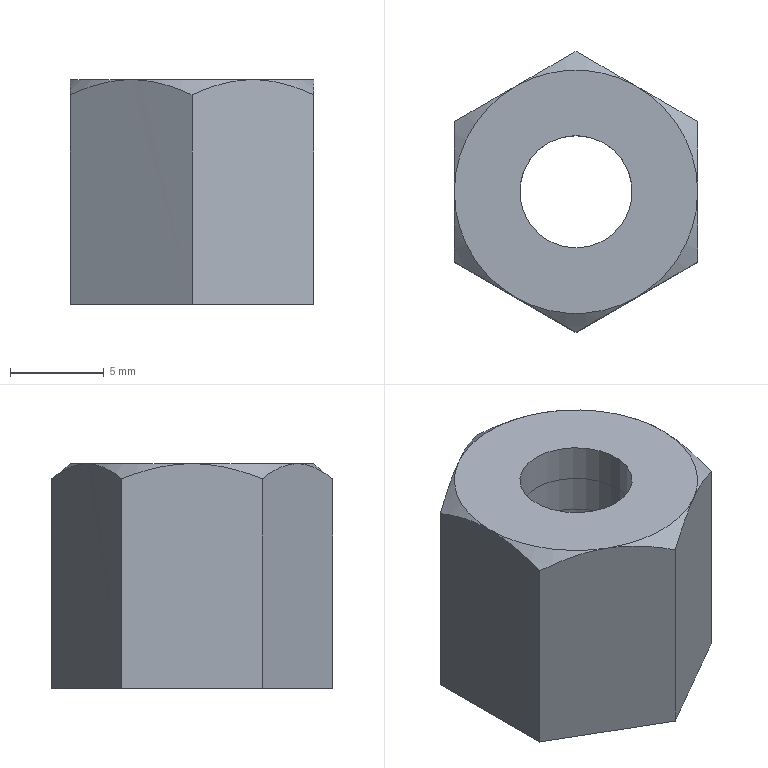Part | STEP file | 1-51.2 | 2 solids | 21 faces | box 13 x 15.011 x 12 mm | volume 1011 mm3 | plane 11 | cone 6 | cylinder 4 | commonest cylinder face diameters 6 x2 10 x2